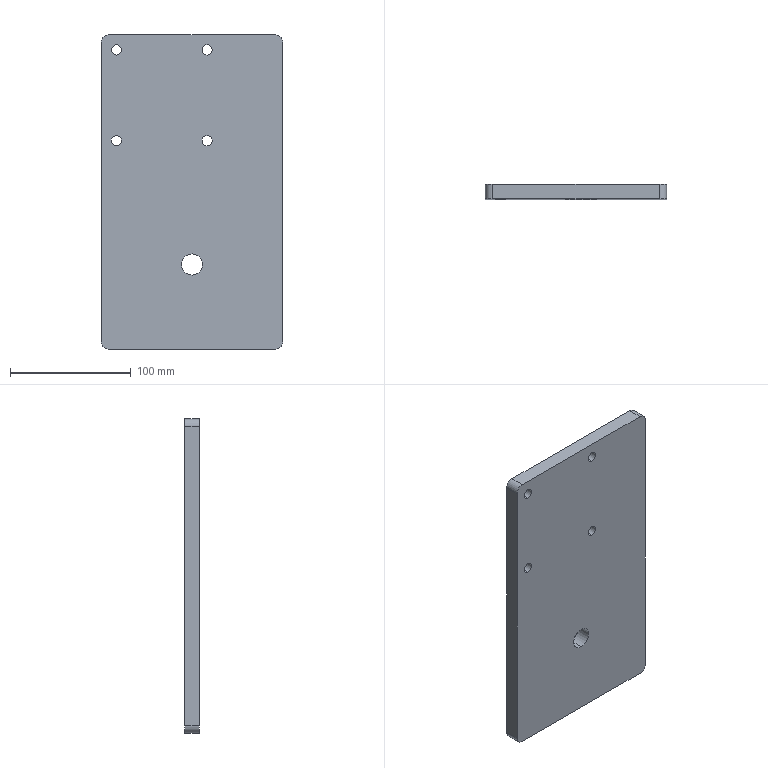Part | SolidWorks | features HoleWzd 2, Extrusion 1, Fillet 1 | 1 solid | 20 faces | box 150 x 12 x 260 mm | volume 462019 mm3 | cylinder 14 | plane 6 | commonest cylinder face diameters 8.5 x8 12 x4 17.5 x2
STEP:
#1=CARTESIAN_POINT('',(-62.5,12.,113.25));
#2=VERTEX_POINT('',#1);
#3=CARTESIAN_POINT('',(-62.5,12.,121.75));
#4=VERTEX_POINT('',#3);
#5=CARTESIAN_POINT('',(-62.5,12.,117.5));
#6=DIRECTION('',(0.,1.,0.));
#7=DIRECTION('',(0.,0.,1.));
#8=AXIS2_PLACEMENT_3D('',#5,#6,#7);
#9=CIRCLE('',#8,4.25);
#10=EDGE_CURVE('',#2,#4,#9,.T.);
#11=ORIENTED_EDGE('',*,*,#10,.T.);
#12=CARTESIAN_POINT('',(-62.5,0.,121.75));
#13=VERTEX_POINT('',#12);
#14=CARTESIAN_POINT('',(-62.5,0.,121.75));
#15=DIRECTION('',(0.,-1.,0.));
#16=VECTOR('',#15,1000.);
#17=LINE('',#14,#16);
#18=EDGE_CURVE('',#4,#13,#17,.T.);
#19=ORIENTED_EDGE('',*,*,#18,.T.);
#20=CARTESIAN_POINT('',(-62.5,0.,113.25));
#21=VERTEX_POINT('',#20);
#22=CARTESIAN_POINT('',(-62.5,0.,117.5));
#23=DIRECTION('',(0.,-1.,0.));
#24=DIRECTION('',(0.,0.,-1.));
#25=AXIS2_PLACEMENT_3D('',#22,#23,#24);
#26=CIRCLE('',#25,4.25);
#27=EDGE_CURVE('',#13,#21,#26,.T.);
#28=ORIENTED_EDGE('',*,*,#27,.T.);
#29=CARTESIAN_POINT('',(-62.5,0.,113.25));
#30=DIRECTION('',(0.,-1.,0.));
#31=VECTOR('',#30,1000.);
#32=LINE('',#29,#31);
#33=EDGE_CURVE('',#2,#21,#32,.T.);
#34=ORIENTED_EDGE('',*,*,#33,.F.);
#35=EDGE_LOOP('',(#11,#19,#28,#34));
#36=FACE_OUTER_BOUND('',#35,.T.);
#37=CARTESIAN_POINT('',(-62.5,0.,117.5));
#38=DIRECTION('',(0.,-1.,0.));
#39=DIRECTION('',(0.,0.,-1.));
#40=AXIS2_PLACEMENT_3D('',#37,#38,#39);
#41=CYLINDRICAL_SURFACE('',#40,4.25);
#42=ADVANCED_FACE('',(#36),#41,.F.);
#43=CARTESIAN_POINT('',(-62.5,12.,38.25));
#44=VERTEX_POINT('',#43);
#45=CARTESIAN_POINT('',(-62.5,12.,46.75));
#46=VERTEX_POINT('',#45);
#47=CARTESIAN_POINT('',(-62.5,12.,42.5));
#48=DIRECTION('',(0.,1.,0.));
#49=DIRECTION('',(0.,0.,1.));
#50=AXIS2_PLACEMENT_3D('',#47,#48,#49);
#51=CIRCLE('',#50,4.25);
#52=EDGE_CURVE('',#44,#46,#51,.T.);
#53=ORIENTED_EDGE('',*,*,#52,.T.);
#54=CARTESIAN_POINT('',(-62.5,0.,46.75));
#55=VERTEX_POINT('',#54);
#56=CARTESIAN_POINT('',(-62.5,0.,46.75));
#57=DIRECTION('',(0.,-1.,0.));
#58=VECTOR('',#57,1000.);
#59=LINE('',#56,#58);
#60=EDGE_CURVE('',#46,#55,#59,.T.);
#61=ORIENTED_EDGE('',*,*,#60,.T.);
#62=CARTESIAN_POINT('',(-62.5,0.,38.25));
#63=VERTEX_POINT('',#62);
#64=CARTESIAN_POINT('',(-62.5,0.,42.5));
#65=DIRECTION('',(0.,-1.,0.));
#66=DIRECTION('',(0.,0.,-1.));
#67=AXIS2_PLACEMENT_3D('',#64,#65,#66);
#68=CIRCLE('',#67,4.25);
#69=EDGE_CURVE('',#55,#63,#68,.T.);
#70=ORIENTED_EDGE('',*,*,#69,.T.);
#71=CARTESIAN_POINT('',(-62.5,0.,38.25));
#72=DIRECTION('',(0.,-1.,0.));
#73=VECTOR('',#72,1000.);
#74=LINE('',#71,#73);
#75=EDGE_CURVE('',#44,#63,#74,.T.);
#76=ORIENTED_EDGE('',*,*,#75,.F.);
#77=EDGE_LOOP('',(#53,#61,#70,#76));
#78=FACE_OUTER_BOUND('',#77,.T.);
#79=CARTESIAN_POINT('',(-62.5,0.,42.5));
#80=DIRECTION('',(0.,-1.,0.));
#81=DIRECTION('',(0.,0.,-1.));
#82=AXIS2_PLACEMENT_3D('',#79,#80,#81);
#83=CYLINDRICAL_SURFACE('',#82,4.25);
#84=ADVANCED_FACE('',(#78),#83,.F.);
#85=CARTESIAN_POINT('',(12.5,12.,38.25));
#86=VERTEX_POINT('',#85);
#87=CARTESIAN_POINT('',(12.5,12.,46.75));
#88=VERTEX_POINT('',#87);
#89=CARTESIAN_POINT('',(12.5,12.,42.5));
#90=DIRECTION('',(0.,1.,0.));
#91=DIRECTION('',(0.,0.,1.));
#92=AXIS2_PLACEMENT_3D('',#89,#90,#91);
#93=CIRCLE('',#92,4.25);
#94=EDGE_CURVE('',#86,#88,#93,.T.);
#95=ORIENTED_EDGE('',*,*,#94,.T.);
#96=CARTESIAN_POINT('',(12.5,0.,46.75));
#97=VERTEX_POINT('',#96);
#98=CARTESIAN_POINT('',(12.5,0.,46.75));
#99=DIRECTION('',(0.,-1.,0.));
#100=VECTOR('',#99,1000.);
#101=LINE('',#98,#100);
#102=EDGE_CURVE('',#88,#97,#101,.T.);
#103=ORIENTED_EDGE('',*,*,#102,.T.);
#104=CARTESIAN_POINT('',(12.5,0.,38.25));
#105=VERTEX_POINT('',#104);
#106=CARTESIAN_POINT('',(12.5,0.,42.5));
#107=DIRECTION('',(0.,-1.,0.));
#108=DIRECTION('',(0.,0.,-1.));
#109=AXIS2_PLACEMENT_3D('',#106,#107,#108);
#110=CIRCLE('',#109,4.25);
#111=EDGE_CURVE('',#97,#105,#110,.T.);
#112=ORIENTED_EDGE('',*,*,#111,.T.);
#113=CARTESIAN_POINT('',(12.5,0.,38.25));
#114=DIRECTION('',(0.,-1.,0.));
#115=VECTOR('',#114,1000.);
#116=LINE('',#113,#115);
#117=EDGE_CURVE('',#86,#105,#116,.T.);
#118=ORIENTED_EDGE('',*,*,#117,.F.);
#119=EDGE_LOOP('',(#95,#103,#112,#118));
#120=FACE_OUTER_BOUND('',#119,.T.);
#121=CARTESIAN_POINT('',(12.5,0.,42.5));
#122=DIRECTION('',(0.,-1.,0.));
#123=DIRECTION('',(0.,0.,-1.));
#124=AXIS2_PLACEMENT_3D('',#121,#122,#123);
#125=CYLINDRICAL_SURFACE('',#124,4.25);
#126=ADVANCED_FACE('',(#120),#125,.F.);
#127=CARTESIAN_POINT('',(12.5,12.,113.25));
#128=VERTEX_POINT('',#127);
#129=CARTESIAN_POINT('',(12.5,12.,121.75));
#130=VERTEX_POINT('',#129);
#131=CARTESIAN_POINT('',(12.5,12.,117.5));
#132=DIRECTION('',(0.,1.,0.));
#133=DIRECTION('',(0.,0.,1.));
#134=AXIS2_PLACEMENT_3D('',#131,#132,#133);
#135=CIRCLE('',#134,4.25);
#136=EDGE_CURVE('',#128,#130,#135,.T.);
#137=ORIENTED_EDGE('',*,*,#136,.T.);
#138=CARTESIAN_POINT('',(12.5,0.,121.75));
#139=VERTEX_POINT('',#138);
#140=CARTESIAN_POINT('',(12.5,0.,121.75));
#141=DIRECTION('',(0.,-1.,0.));
#142=VECTOR('',#141,1000.);
#143=LINE('',#140,#142);
#144=EDGE_CURVE('',#130,#139,#143,.T.);
#145=ORIENTED_EDGE('',*,*,#144,.T.);
#146=CARTESIAN_POINT('',(12.5,0.,113.25));
#147=VERTEX_POINT('',#146);
#148=CARTESIAN_POINT('',(12.5,0.,117.5));
#149=DIRECTION('',(0.,-1.,0.));
#150=DIRECTION('',(0.,0.,-1.));
#151=AXIS2_PLACEMENT_3D('',#148,#149,#150);
#152=CIRCLE('',#151,4.25);
#153=EDGE_CURVE('',#139,#147,#152,.T.);
#154=ORIENTED_EDGE('',*,*,#153,.T.);
#155=CARTESIAN_POINT('',(12.5,0.,113.25));
#156=DIRECTION('',(0.,-1.,0.));
#157=VECTOR('',#156,1000.);
#158=LINE('',#155,#157);
#159=EDGE_CURVE('',#128,#147,#158,.T.);
#160=ORIENTED_EDGE('',*,*,#159,.F.);
#161=EDGE_LOOP('',(#137,#145,#154,#160));
#162=FACE_OUTER_BOUND('',#161,.T.);
#163=CARTESIAN_POINT('',(12.5,0.,117.5));
#164=DIRECTION('',(0.,-1.,0.));
#165=DIRECTION('',(0.,0.,-1.));
#166=AXIS2_PLACEMENT_3D('',#163,#164,#165);
#167=CYLINDRICAL_SURFACE('',#166,4.25);
#168=ADVANCED_FACE('',(#162),#167,.F.);
#169=CARTESIAN_POINT('',(0.,12.,-68.75));
#170=VERTEX_POINT('',#169);
#171=CARTESIAN_POINT('',(0.,12.,-51.25));
#172=VERTEX_POINT('',#171);
#173=CARTESIAN_POINT('',(0.,12.,-60.));
#174=DIRECTION('',(0.,1.,0.));
#175=DIRECTION('',(0.,0.,1.));
#176=AXIS2_PLACEMENT_3D('',#173,#174,#175);
#177=CIRCLE('',#176,8.75);
#178=EDGE_CURVE('',#170,#172,#177,.T.);
#179=ORIENTED_EDGE('',*,*,#178,.T.);
#180=CARTESIAN_POINT('',(0.,0.,-51.25));
#181=VERTEX_POINT('',#180);
#182=CARTESIAN_POINT('',(0.,0.,-51.25));
#183=DIRECTION('',(0.,-1.,0.));
#184=VECTOR('',#183,1000.);
#185=LINE('',#182,#184);
#186=EDGE_CURVE('',#172,#181,#185,.T.);
#187=ORIENTED_EDGE('',*,*,#186,.T.);
#188=CARTESIAN_POINT('',(0.,0.,-68.75));
#189=VERTEX_POINT('',#188);
#190=CARTESIAN_POINT('',(0.,0.,-60.));
#191=DIRECTION('',(0.,-1.,0.));
#192=DIRECTION('',(0.,0.,-1.));
#193=AXIS2_PLACEMENT_3D('',#190,#191,#192);
#194=CIRCLE('',#193,8.75);
#195=EDGE_CURVE('',#181,#189,#194,.T.);
#196=ORIENTED_EDGE('',*,*,#195,.T.);
#197=CARTESIAN_POINT('',(0.,0.,-68.75));
#198=DIRECTION('',(0.,-1.,0.));
#199=VECTOR('',#198,1000.);
#200=LINE('',#197,#199);
#201=EDGE_CURVE('',#170,#189,#200,.T.);
#202=ORIENTED_EDGE('',*,*,#201,.F.);
#203=EDGE_LOOP('',(#179,#187,#196,#202));
#204=FACE_OUTER_BOUND('',#203,.T.);
#205=CARTESIAN_POINT('',(0.,0.,-60.));
#206=DIRECTION('',(0.,-1.,0.));
#207=DIRECTION('',(0.,0.,-1.));
#208=AXIS2_PLACEMENT_3D('',#205,#206,#207);
#209=CYLINDRICAL_SURFACE('',#208,8.75);
#210=ADVANCED_FACE('',(#204),#209,.F.);
#211=CARTESIAN_POINT('',(-62.5,0.,117.5));
#212=DIRECTION('',(0.,-1.,0.));
#213=DIRECTION('',(0.,0.,-1.));
#214=AXIS2_PLACEMENT_3D('',#211,#212,#213);
#215=CIRCLE('',#214,4.25);
#216=EDGE_CURVE('',#21,#13,#215,.T.);
#217=ORIENTED_EDGE('',*,*,#216,.F.);
#218=ORIENTED_EDGE('',*,*,#27,.F.);
#219=EDGE_LOOP('',(#217,#218));
#220=FACE_BOUND('',#219,.T.);
#221=CARTESIAN_POINT('',(12.5,0.,42.5));
#222=DIRECTION('',(0.,-1.,0.));
#223=DIRECTION('',(0.,0.,-1.));
#224=AXIS2_PLACEMENT_3D('',#221,#222,#223);
#225=CIRCLE('',#224,4.25);
#226=EDGE_CURVE('',#105,#97,#225,.T.);
#227=ORIENTED_EDGE('',*,*,#226,.F.);
#228=ORIENTED_EDGE('',*,*,#111,.F.);
#229=EDGE_LOOP('',(#227,#228));
#230=FACE_BOUND('',#229,.T.);
#231=CARTESIAN_POINT('',(12.5,0.,117.5));
#232=DIRECTION('',(0.,-1.,0.));
#233=DIRECTION('',(0.,0.,-1.));
#234=AXIS2_PLACEMENT_3D('',#231,#232,#233);
#235=CIRCLE('',#234,4.25);
#236=EDGE_CURVE('',#147,#139,#235,.T.);
#237=ORIENTED_EDGE('',*,*,#236,.F.);
#238=ORIENTED_EDGE('',*,*,#153,.F.);
#239=EDGE_LOOP('',(#237,#238));
#240=FACE_BOUND('',#239,.T.);
#241=CARTESIAN_POINT('',(0.,0.,-60.));
#242=DIRECTION('',(0.,-1.,0.));
#243=DIRECTION('',(0.,0.,-1.));
#244=AXIS2_PLACEMENT_3D('',#241,#242,#243);
#245=CIRCLE('',#244,8.75);
#246=EDGE_CURVE('',#189,#181,#245,.T.);
#247=ORIENTED_EDGE('',*,*,#246,.F.);
#248=ORIENTED_EDGE('',*,*,#195,.F.);
#249=EDGE_LOOP('',(#247,#248));
#250=FACE_BOUND('',#249,.T.);
#251=CARTESIAN_POINT('',(69.,0.,-130.));
#252=VERTEX_POINT('',#251);
#253=CARTESIAN_POINT('',(-69.,0.,-130.));
#254=VERTEX_POINT('',#253);
#255=CARTESIAN_POINT('',(-75.,0.,-130.));
#256=DIRECTION('',(-1.,0.,0.));
#257=VECTOR('',#256,1000.);
#258=LINE('',#255,#257);
#259=EDGE_CURVE('',#252,#254,#258,.T.);
#260=ORIENTED_EDGE('',*,*,#259,.F.);
#261=CARTESIAN_POINT('',(75.,0.,-124.));
#262=VERTEX_POINT('',#261);
#263=CARTESIAN_POINT('',(69.,0.,-124.));
#264=DIRECTION('',(0.,-1.,0.));
#265=DIRECTION('',(0.,0.,1.));
#266=AXIS2_PLACEMENT_3D('',#263,#264,#265);
#267=CIRCLE('',#266,6.);
#268=EDGE_CURVE('',#252,#262,#267,.T.);
#269=ORIENTED_EDGE('',*,*,#268,.T.);
#270=CARTESIAN_POINT('',(75.,0.,124.));
#271=VERTEX_POINT('',#270);
#272=CARTESIAN_POINT('',(75.,0.,-130.));
#273=DIRECTION('',(0.,0.,-1.));
#274=VECTOR('',#273,1000.);
#275=LINE('',#272,#274);
#276=EDGE_CURVE('',#271,#262,#275,.T.);
#277=ORIENTED_EDGE('',*,*,#276,.F.);
#278=CARTESIAN_POINT('',(69.,0.,130.));
#279=VERTEX_POINT('',#278);
#280=CARTESIAN_POINT('',(69.,0.,124.));
#281=DIRECTION('',(0.,-1.,0.));
#282=DIRECTION('',(0.,0.,1.));
#283=AXIS2_PLACEMENT_3D('',#280,#281,#282);
#284=CIRCLE('',#283,6.);
#285=EDGE_CURVE('',#271,#279,#284,.T.);
#286=ORIENTED_EDGE('',*,*,#285,.T.);
#287=CARTESIAN_POINT('',(-69.,0.,130.));
#288=VERTEX_POINT('',#287);
#289=CARTESIAN_POINT('',(-75.,0.,130.));
#290=DIRECTION('',(1.,0.,0.));
#291=VECTOR('',#290,1000.);
#292=LINE('',#289,#291);
#293=EDGE_CURVE('',#288,#279,#292,.T.);
#294=ORIENTED_EDGE('',*,*,#293,.F.);
#295=CARTESIAN_POINT('',(-75.,0.,124.));
#296=VERTEX_POINT('',#295);
#297=CARTESIAN_POINT('',(-69.,0.,124.));
#298=DIRECTION('',(0.,-1.,0.));
#299=DIRECTION('',(0.,0.,1.));
#300=AXIS2_PLACEMENT_3D('',#297,#298,#299);
#301=CIRCLE('',#300,6.);
#302=EDGE_CURVE('',#288,#296,#301,.T.);
#303=ORIENTED_EDGE('',*,*,#302,.T.);
#304=CARTESIAN_POINT('',(-75.,0.,-124.));
#305=VERTEX_POINT('',#304);
#306=CARTESIAN_POINT('',(-75.,0.,-130.));
#307=DIRECTION('',(0.,0.,1.));
#308=VECTOR('',#307,1000.);
#309=LINE('',#306,#308);
#310=EDGE_CURVE('',#305,#296,#309,.T.);
#311=ORIENTED_EDGE('',*,*,#310,.F.);
#312=CARTESIAN_POINT('',(-69.,0.,-124.));
#313=DIRECTION('',(0.,-1.,0.));
#314=DIRECTION('',(0.,0.,1.));
#315=AXIS2_PLACEMENT_3D('',#312,#313,#314);
#316=CIRCLE('',#315,6.);
#317=EDGE_CURVE('',#305,#254,#316,.T.);
#318=ORIENTED_EDGE('',*,*,#317,.T.);
#319=EDGE_LOOP('',(#260,#269,#277,#286,#294,#303,#311,#318));
#320=FACE_OUTER_BOUND('',#319,.T.);
#321=CARTESIAN_POINT('',(-62.5,0.,42.5));
#322=DIRECTION('',(0.,-1.,0.));
#323=DIRECTION('',(0.,0.,-1.));
#324=AXIS2_PLACEMENT_3D('',#321,#322,#323);
#325=CIRCLE('',#324,4.25);
#326=EDGE_CURVE('',#63,#55,#325,.T.);
#327=ORIENTED_EDGE('',*,*,#326,.F.);
#328=ORIENTED_EDGE('',*,*,#69,.F.);
#329=EDGE_LOOP('',(#327,#328));
#330=FACE_BOUND('',#329,.T.);
#331=CARTESIAN_POINT('',(0.,0.,0.));
#332=DIRECTION('',(0.,1.,0.));
#333=DIRECTION('',(0.,0.,1.));
#334=AXIS2_PLACEMENT_3D('',#331,#332,#333);
#335=PLANE('',#334);
#336=ADVANCED_FACE('',(#220,#230,#240,#250,#320,#330),#335,.F.);
#337=ORIENTED_EDGE('',*,*,#276,.T.);
#338=CARTESIAN_POINT('',(75.,12.,-124.));
#339=VERTEX_POINT('',#338);
#340=CARTESIAN_POINT('',(75.,12.,-124.));
#341=DIRECTION('',(0.,1.,0.));
#342=VECTOR('',#341,1000.);
#343=LINE('',#340,#342);
#344=EDGE_CURVE('',#262,#339,#343,.T.);
#345=ORIENTED_EDGE('',*,*,#344,.T.);
#346=CARTESIAN_POINT('',(75.,12.,124.));
#347=VERTEX_POINT('',#346);
#348=CARTESIAN_POINT('',(75.,12.,-130.));
#349=DIRECTION('',(0.,0.,-1.));
#350=VECTOR('',#349,1000.);
#351=LINE('',#348,#350);
#352=EDGE_CURVE('',#347,#339,#351,.T.);
#353=ORIENTED_EDGE('',*,*,#352,.F.);
#354=CARTESIAN_POINT('',(75.,12.,124.));
#355=DIRECTION('',(0.,-1.,0.));
#356=VECTOR('',#355,1000.);
#357=LINE('',#354,#356);
#358=EDGE_CURVE('',#347,#271,#357,.T.);
#359=ORIENTED_EDGE('',*,*,#358,.T.);
#360=EDGE_LOOP('',(#337,#345,#353,#359));
#361=FACE_OUTER_BOUND('',#360,.T.);
#362=CARTESIAN_POINT('',(75.,12.,-130.));
#363=DIRECTION('',(-1.,0.,0.));
#364=DIRECTION('',(0.,0.,1.));
#365=AXIS2_PLACEMENT_3D('',#362,#363,#364);
#366=PLANE('',#365);
#367=ADVANCED_FACE('',(#361),#366,.F.);
#368=CARTESIAN_POINT('',(69.,12.,-130.));
#369=VERTEX_POINT('',#368);
#370=CARTESIAN_POINT('',(-69.,12.,-130.));
#371=VERTEX_POINT('',#370);
#372=CARTESIAN_POINT('',(-75.,12.,-130.));
#373=DIRECTION('',(-1.,0.,0.));
#374=VECTOR('',#373,1000.);
#375=LINE('',#372,#374);
#376=EDGE_CURVE('',#369,#371,#375,.T.);
#377=ORIENTED_EDGE('',*,*,#376,.F.);
#378=CARTESIAN_POINT('',(69.,12.,-130.));
#379=DIRECTION('',(0.,-1.,0.));
#380=VECTOR('',#379,1000.);
#381=LINE('',#378,#380);
#382=EDGE_CURVE('',#369,#252,#381,.T.);
#383=ORIENTED_EDGE('',*,*,#382,.T.);
#384=ORIENTED_EDGE('',*,*,#259,.T.);
#385=CARTESIAN_POINT('',(-69.,12.,-130.));
#386=DIRECTION('',(0.,1.,0.));
#387=VECTOR('',#386,1000.);
#388=LINE('',#385,#387);
#389=EDGE_CURVE('',#254,#371,#388,.T.);
#390=ORIENTED_EDGE('',*,*,#389,.T.);
#391=EDGE_LOOP('',(#377,#383,#384,#390));
#392=FACE_OUTER_BOUND('',#391,.T.);
#393=CARTESIAN_POINT('',(-75.,12.,-130.));
#394=DIRECTION('',(0.,0.,1.));
#395=DIRECTION('',(1.,0.,0.));
#396=AXIS2_PLACEMENT_3D('',#393,#394,#395);
#397=PLANE('',#396);
#398=ADVANCED_FACE('',(#392),#397,.F.);
#399=ORIENTED_EDGE('',*,*,#310,.T.);
#400=CARTESIAN_POINT('',(-75.,12.,124.));
#401=VERTEX_POINT('',#400);
#402=CARTESIAN_POINT('',(-75.,12.,124.));
#403=DIRECTION('',(0.,1.,0.));
#404=VECTOR('',#403,1000.);
#405=LINE('',#402,#404);
#406=EDGE_CURVE('',#296,#401,#405,.T.);
#407=ORIENTED_EDGE('',*,*,#406,.T.);
#408=CARTESIAN_POINT('',(-75.,12.,-124.));
#409=VERTEX_POINT('',#408);
#410=CARTESIAN_POINT('',(-75.,12.,-130.));
#411=DIRECTION('',(0.,0.,1.));
#412=VECTOR('',#411,1000.);
#413=LINE('',#410,#412);
#414=EDGE_CURVE('',#409,#401,#413,.T.);
#415=ORIENTED_EDGE('',*,*,#414,.F.);
#416=CARTESIAN_POINT('',(-75.,12.,-124.));
#417=DIRECTION('',(0.,-1.,0.));
#418=VECTOR('',#417,1000.);
#419=LINE('',#416,#418);
#420=EDGE_CURVE('',#409,#305,#419,.T.);
#421=ORIENTED_EDGE('',*,*,#420,.T.);
#422=EDGE_LOOP('',(#399,#407,#415,#421));
#423=FACE_OUTER_BOUND('',#422,.T.);
#424=CARTESIAN_POINT('',(-75.,12.,-130.));
#425=DIRECTION('',(1.,0.,0.));
#426=DIRECTION('',(0.,0.,-1.));
#427=AXIS2_PLACEMENT_3D('',#424,#425,#426);
#428=PLANE('',#427);
#429=ADVANCED_FACE('',(#423),#428,.F.);
#430=ORIENTED_EDGE('',*,*,#293,.T.);
#431=CARTESIAN_POINT('',(69.,12.,130.));
#432=VERTEX_POINT('',#431);
#433=CARTESIAN_POINT('',(69.,12.,130.));
#434=DIRECTION('',(0.,1.,0.));
#435=VECTOR('',#434,1000.);
#436=LINE('',#433,#435);
#437=EDGE_CURVE('',#279,#432,#436,.T.);
#438=ORIENTED_EDGE('',*,*,#437,.T.);
#439=CARTESIAN_POINT('',(-69.,12.,130.));
#440=VERTEX_POINT('',#439);
#441=CARTESIAN_POINT('',(-75.,12.,130.));
#442=DIRECTION('',(1.,0.,0.));
#443=VECTOR('',#442,1000.);
#444=LINE('',#441,#443);
#445=EDGE_CURVE('',#440,#432,#444,.T.);
#446=ORIENTED_EDGE('',*,*,#445,.F.);
#447=CARTESIAN_POINT('',(-69.,12.,130.));
#448=DIRECTION('',(0.,-1.,0.));
#449=VECTOR('',#448,1000.);
#450=LINE('',#447,#449);
#451=EDGE_CURVE('',#440,#288,#450,.T.);
#452=ORIENTED_EDGE('',*,*,#451,.T.);
#453=EDGE_LOOP('',(#430,#438,#446,#452));
#454=FACE_OUTER_BOUND('',#453,.T.);
#455=CARTESIAN_POINT('',(-75.,12.,130.));
#456=DIRECTION('',(0.,0.,-1.));
#457=DIRECTION('',(-1.,0.,0.));
#458=AXIS2_PLACEMENT_3D('',#455,#456,#457);
#459=PLANE('',#458);
#460=ADVANCED_FACE('',(#454),#459,.F.);
#461=ORIENTED_EDGE('',*,*,#10,.F.);
#462=CARTESIAN_POINT('',(-62.5,12.,117.5));
#463=DIRECTION('',(0.,1.,0.));
#464=DIRECTION('',(0.,0.,1.));
#465=AXIS2_PLACEMENT_3D('',#462,#463,#464);
#466=CIRCLE('',#465,4.25);
#467=EDGE_CURVE('',#4,#2,#466,.T.);
#468=ORIENTED_EDGE('',*,*,#467,.F.);
#469=EDGE_LOOP('',(#461,#468));
#470=FACE_BOUND('',#469,.T.);
#471=ORIENTED_EDGE('',*,*,#52,.F.);
#472=CARTESIAN_POINT('',(-62.5,12.,42.5));
#473=DIRECTION('',(0.,1.,0.));
#474=DIRECTION('',(0.,0.,1.));
#475=AXIS2_PLACEMENT_3D('',#472,#473,#474);
#476=CIRCLE('',#475,4.25);
#477=EDGE_CURVE('',#46,#44,#476,.T.);
#478=ORIENTED_EDGE('',*,*,#477,.F.);
#479=EDGE_LOOP('',(#471,#478));
#480=FACE_BOUND('',#479,.T.);
#481=ORIENTED_EDGE('',*,*,#94,.F.);
#482=CARTESIAN_POINT('',(12.5,12.,42.5));
#483=DIRECTION('',(0.,1.,0.));
#484=DIRECTION('',(0.,0.,1.));
#485=AXIS2_PLACEMENT_3D('',#482,#483,#484);
#486=CIRCLE('',#485,4.25);
#487=EDGE_CURVE('',#88,#86,#486,.T.);
#488=ORIENTED_EDGE('',*,*,#487,.F.);
#489=EDGE_LOOP('',(#481,#488));
#490=FACE_BOUND('',#489,.T.);
#491=ORIENTED_EDGE('',*,*,#136,.F.);
#492=CARTESIAN_POINT('',(12.5,12.,117.5));
#493=DIRECTION('',(0.,1.,0.));
#494=DIRECTION('',(0.,0.,1.));
#495=AXIS2_PLACEMENT_3D('',#492,#493,#494);
#496=CIRCLE('',#495,4.25);
#497=EDGE_CURVE('',#130,#128,#496,.T.);
#498=ORIENTED_EDGE('',*,*,#497,.F.);
#499=EDGE_LOOP('',(#491,#498));
#500=FACE_BOUND('',#499,.T.);
#501=ORIENTED_EDGE('',*,*,#178,.F.);
#502=CARTESIAN_POINT('',(0.,12.,-60.));
#503=DIRECTION('',(0.,1.,0.));
#504=DIRECTION('',(0.,0.,1.));
#505=AXIS2_PLACEMENT_3D('',#502,#503,#504);
#506=CIRCLE('',#505,8.75);
#507=EDGE_CURVE('',#172,#170,#506,.T.);
#508=ORIENTED_EDGE('',*,*,#507,.F.);
#509=EDGE_LOOP('',(#501,#508));
#510=FACE_BOUND('',#509,.T.);
#511=ORIENTED_EDGE('',*,*,#352,.T.);
#512=CARTESIAN_POINT('',(69.,12.,-124.));
#513=DIRECTION('',(0.,1.,0.));
#514=DIRECTION('',(0.,0.,1.));
#515=AXIS2_PLACEMENT_3D('',#512,#513,#514);
#516=CIRCLE('',#515,6.);
#517=EDGE_CURVE('',#339,#369,#516,.T.);
#518=ORIENTED_EDGE('',*,*,#517,.T.);
#519=ORIENTED_EDGE('',*,*,#376,.T.);
#520=CARTESIAN_POINT('',(-69.,12.,-124.));
#521=DIRECTION('',(0.,1.,0.));
#522=DIRECTION('',(0.,0.,1.));
#523=AXIS2_PLACEMENT_3D('',#520,#521,#522);
#524=CIRCLE('',#523,6.);
#525=EDGE_CURVE('',#371,#409,#524,.T.);
#526=ORIENTED_EDGE('',*,*,#525,.T.);
#527=ORIENTED_EDGE('',*,*,#414,.T.);
#528=CARTESIAN_POINT('',(-69.,12.,124.));
#529=DIRECTION('',(0.,1.,0.));
#530=DIRECTION('',(0.,0.,1.));
#531=AXIS2_PLACEMENT_3D('',#528,#529,#530);
#532=CIRCLE('',#531,6.);
#533=EDGE_CURVE('',#401,#440,#532,.T.);
#534=ORIENTED_EDGE('',*,*,#533,.T.);
#535=ORIENTED_EDGE('',*,*,#445,.T.);
#536=CARTESIAN_POINT('',(69.,12.,124.));
#537=DIRECTION('',(0.,1.,0.));
#538=DIRECTION('',(0.,0.,1.));
#539=AXIS2_PLACEMENT_3D('',#536,#537,#538);
#540=CIRCLE('',#539,6.);
#541=EDGE_CURVE('',#432,#347,#540,.T.);
#542=ORIENTED_EDGE('',*,*,#541,.T.);
#543=EDGE_LOOP('',(#511,#518,#519,#526,#527,#534,#535,#542));
#544=FACE_OUTER_BOUND('',#543,.T.);
#545=CARTESIAN_POINT('',(0.,12.,0.));
#546=DIRECTION('',(0.,1.,0.));
#547=DIRECTION('',(0.,0.,1.));
#548=AXIS2_PLACEMENT_3D('',#545,#546,#547);
#549=PLANE('',#548);
#550=ADVANCED_FACE('',(#470,#480,#490,#500,#510,#544),#549,.T.);
#551=ORIENTED_EDGE('',*,*,#517,.F.);
#552=ORIENTED_EDGE('',*,*,#344,.F.);
#553=ORIENTED_EDGE('',*,*,#268,.F.);
#554=ORIENTED_EDGE('',*,*,#382,.F.);
#555=EDGE_LOOP('',(#551,#552,#553,#554));
#556=FACE_OUTER_BOUND('',#555,.T.);
#557=CARTESIAN_POINT('',(69.,12.,-124.));
#558=DIRECTION('',(0.,-1.,0.));
#559=DIRECTION('',(0.,0.,-1.));
#560=AXIS2_PLACEMENT_3D('',#557,#558,#559);
#561=CYLINDRICAL_SURFACE('',#560,6.);
#562=ADVANCED_FACE('',(#556),#561,.T.);
#563=ORIENTED_EDGE('',*,*,#541,.F.);
#564=ORIENTED_EDGE('',*,*,#437,.F.);
#565=ORIENTED_EDGE('',*,*,#285,.F.);
#566=ORIENTED_EDGE('',*,*,#358,.F.);
#567=EDGE_LOOP('',(#563,#564,#565,#566));
#568=FACE_OUTER_BOUND('',#567,.T.);
#569=CARTESIAN_POINT('',(69.,12.,124.));
#570=DIRECTION('',(0.,-1.,0.));
#571=DIRECTION('',(0.,0.,-1.));
#572=AXIS2_PLACEMENT_3D('',#569,#570,#571);
#573=CYLINDRICAL_SURFACE('',#572,6.);
#574=ADVANCED_FACE('',(#568),#573,.T.);
#575=ORIENTED_EDGE('',*,*,#533,.F.);
#576=ORIENTED_EDGE('',*,*,#406,.F.);
#577=ORIENTED_EDGE('',*,*,#302,.F.);
#578=ORIENTED_EDGE('',*,*,#451,.F.);
#579=EDGE_LOOP('',(#575,#576,#577,#578));
#580=FACE_OUTER_BOUND('',#579,.T.);
#581=CARTESIAN_POINT('',(-69.,12.,124.));
#582=DIRECTION('',(0.,-1.,0.));
#583=DIRECTION('',(0.,0.,-1.));
#584=AXIS2_PLACEMENT_3D('',#581,#582,#583);
#585=CYLINDRICAL_SURFACE('',#584,6.);
#586=ADVANCED_FACE('',(#580),#585,.T.);
#587=ORIENTED_EDGE('',*,*,#525,.F.);
#588=ORIENTED_EDGE('',*,*,#389,.F.);
#589=ORIENTED_EDGE('',*,*,#317,.F.);
#590=ORIENTED_EDGE('',*,*,#420,.F.);
#591=EDGE_LOOP('',(#587,#588,#589,#590));
#592=FACE_OUTER_BOUND('',#591,.T.);
#593=CARTESIAN_POINT('',(-69.,12.,-124.));
#594=DIRECTION('',(0.,-1.,0.));
#595=DIRECTION('',(0.,0.,-1.));
#596=AXIS2_PLACEMENT_3D('',#593,#594,#595);
#597=CYLINDRICAL_SURFACE('',#596,6.);
#598=ADVANCED_FACE('',(#592),#597,.T.);
#599=ORIENTED_EDGE('',*,*,#186,.F.);
#600=ORIENTED_EDGE('',*,*,#507,.T.);
#601=ORIENTED_EDGE('',*,*,#201,.T.);
#602=ORIENTED_EDGE('',*,*,#246,.T.);
#603=EDGE_LOOP('',(#599,#600,#601,#602));
#604=FACE_OUTER_BOUND('',#603,.T.);
#605=CARTESIAN_POINT('',(0.,0.,-60.));
#606=DIRECTION('',(0.,-1.,0.));
#607=DIRECTION('',(0.,0.,-1.));
#608=AXIS2_PLACEMENT_3D('',#605,#606,#607);
#609=CYLINDRICAL_SURFACE('',#608,8.75);
#610=ADVANCED_FACE('',(#604),#609,.F.);
#611=ORIENTED_EDGE('',*,*,#144,.F.);
#612=ORIENTED_EDGE('',*,*,#497,.T.);
#613=ORIENTED_EDGE('',*,*,#159,.T.);
#614=ORIENTED_EDGE('',*,*,#236,.T.);
#615=EDGE_LOOP('',(#611,#612,#613,#614));
#616=FACE_OUTER_BOUND('',#615,.T.);
#617=CARTESIAN_POINT('',(12.5,0.,117.5));
#618=DIRECTION('',(0.,-1.,0.));
#619=DIRECTION('',(0.,0.,-1.));
#620=AXIS2_PLACEMENT_3D('',#617,#618,#619);
#621=CYLINDRICAL_SURFACE('',#620,4.25);
#622=ADVANCED_FACE('',(#616),#621,.F.);
#623=ORIENTED_EDGE('',*,*,#102,.F.);
#624=ORIENTED_EDGE('',*,*,#487,.T.);
#625=ORIENTED_EDGE('',*,*,#117,.T.);
#626=ORIENTED_EDGE('',*,*,#226,.T.);
#627=EDGE_LOOP('',(#623,#624,#625,#626));
#628=FACE_OUTER_BOUND('',#627,.T.);
#629=CARTESIAN_POINT('',(12.5,0.,42.5));
#630=DIRECTION('',(0.,-1.,0.));
#631=DIRECTION('',(0.,0.,-1.));
#632=AXIS2_PLACEMENT_3D('',#629,#630,#631);
#633=CYLINDRICAL_SURFACE('',#632,4.25);
#634=ADVANCED_FACE('',(#628),#633,.F.);
#635=ORIENTED_EDGE('',*,*,#60,.F.);
#636=ORIENTED_EDGE('',*,*,#477,.T.);
#637=ORIENTED_EDGE('',*,*,#75,.T.);
#638=ORIENTED_EDGE('',*,*,#326,.T.);
#639=EDGE_LOOP('',(#635,#636,#637,#638));
#640=FACE_OUTER_BOUND('',#639,.T.);
#641=CARTESIAN_POINT('',(-62.5,0.,42.5));
#642=DIRECTION('',(0.,-1.,0.));
#643=DIRECTION('',(0.,0.,-1.));
#644=AXIS2_PLACEMENT_3D('',#641,#642,#643);
#645=CYLINDRICAL_SURFACE('',#644,4.25);
#646=ADVANCED_FACE('',(#640),#645,.F.);
#647=ORIENTED_EDGE('',*,*,#18,.F.);
#648=ORIENTED_EDGE('',*,*,#467,.T.);
#649=ORIENTED_EDGE('',*,*,#33,.T.);
#650=ORIENTED_EDGE('',*,*,#216,.T.);
#651=EDGE_LOOP('',(#647,#648,#649,#650));
#652=FACE_OUTER_BOUND('',#651,.T.);
#653=CARTESIAN_POINT('',(-62.5,0.,117.5));
#654=DIRECTION('',(0.,-1.,0.));
#655=DIRECTION('',(0.,0.,-1.));
#656=AXIS2_PLACEMENT_3D('',#653,#654,#655);
#657=CYLINDRICAL_SURFACE('',#656,4.25);
#658=ADVANCED_FACE('',(#652),#657,.F.);
#659=CLOSED_SHELL('',(#42,#84,#126,#168,#210,#336,#367,#398,#429,#460,#550,#562,#574,#586,#598,#610,#622,#634,#646,#658));
#660=MANIFOLD_SOLID_BREP('',#659);
#661=CARTESIAN_POINT('',(0.,0.,0.));
#662=DIRECTION('',(0.,0.,1.));
#663=DIRECTION('',(1.,0.,0.));
#664=AXIS2_PLACEMENT_3D('',#661,#662,#663);
#665=(LENGTH_UNIT()NAMED_UNIT(*)SI_UNIT(.MILLI.,.METRE.));
#666=UNCERTAINTY_MEASURE_WITH_UNIT(LENGTH_MEASURE(0.00001),#665,'','');
#667=(NAMED_UNIT(*)PLANE_ANGLE_UNIT()SI_UNIT($,.RADIAN.));
#668=(NAMED_UNIT(*)SI_UNIT($,.STERADIAN.)SOLID_ANGLE_UNIT());
#669=(GEOMETRIC_REPRESENTATION_CONTEXT(3)GLOBAL_UNCERTAINTY_ASSIGNED_CONTEXT((#666))GLOBAL_UNIT_ASSIGNED_CONTEXT((#665,#667,#668))REPRESENTATION_CONTEXT('',''));
#670=ADVANCED_BREP_SHAPE_REPRESENTATION('',(#660,#664),#669);